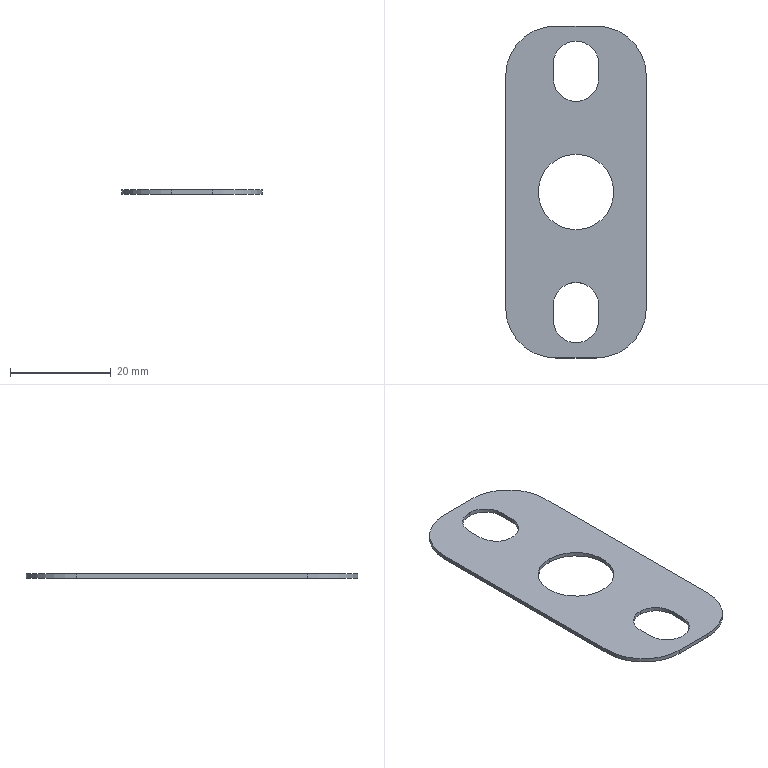Part | SolidWorks | features BaseBody 1 | 1 solid | 22 faces | box 28 x 66 x 0.8 mm | volume 1123 mm3 | cylinder 12 | plane 10 | commonest cylinder face diameters 9 x6 20 x4 15 x2
STEP:
#1=CARTESIAN_POINT('',(172.5,7.5,46.));
#2=VERTEX_POINT('',#1);
#3=CARTESIAN_POINT('',(172.5,-7.5,46.));
#4=VERTEX_POINT('',#3);
#5=CARTESIAN_POINT('',(172.5,0.,46.));
#6=DIRECTION('',(0.,0.,-1.));
#7=DIRECTION('',(0.,-1.,0.));
#8=AXIS2_PLACEMENT_3D('',#5,#6,#7);
#9=CIRCLE('',#8,7.5);
#10=EDGE_CURVE('',#2,#4,#9,.T.);
#11=ORIENTED_EDGE('',*,*,#10,.T.);
#12=CARTESIAN_POINT('',(172.5,-7.5,46.8));
#13=VERTEX_POINT('',#12);
#14=CARTESIAN_POINT('',(172.5,-7.5,46.));
#15=DIRECTION('',(0.,0.,1.));
#16=VECTOR('',#15,1000.);
#17=LINE('',#14,#16);
#18=EDGE_CURVE('',#4,#13,#17,.T.);
#19=ORIENTED_EDGE('',*,*,#18,.T.);
#20=CARTESIAN_POINT('',(172.5,7.5,46.8));
#21=VERTEX_POINT('',#20);
#22=CARTESIAN_POINT('',(172.5,0.,46.8));
#23=DIRECTION('',(0.,0.,-1.));
#24=DIRECTION('',(0.,-1.,0.));
#25=AXIS2_PLACEMENT_3D('',#22,#23,#24);
#26=CIRCLE('',#25,7.5);
#27=EDGE_CURVE('',#21,#13,#26,.T.);
#28=ORIENTED_EDGE('',*,*,#27,.F.);
#29=CARTESIAN_POINT('',(172.5,7.5,46.));
#30=DIRECTION('',(0.,0.,1.));
#31=VECTOR('',#30,1000.);
#32=LINE('',#29,#31);
#33=EDGE_CURVE('',#2,#21,#32,.T.);
#34=ORIENTED_EDGE('',*,*,#33,.F.);
#35=EDGE_LOOP('',(#11,#19,#28,#34));
#36=FACE_OUTER_BOUND('',#35,.T.);
#37=CARTESIAN_POINT('',(172.5,0.,46.));
#38=DIRECTION('',(0.,0.,1.));
#39=DIRECTION('',(0.,1.,0.));
#40=AXIS2_PLACEMENT_3D('',#37,#38,#39);
#41=CYLINDRICAL_SURFACE('',#40,7.5);
#42=ADVANCED_FACE('',(#36),#41,.F.);
#43=CARTESIAN_POINT('',(168.,25.5,46.));
#44=VERTEX_POINT('',#43);
#45=CARTESIAN_POINT('',(172.5,30.,46.));
#46=VERTEX_POINT('',#45);
#47=CARTESIAN_POINT('',(172.5,25.5,46.));
#48=DIRECTION('',(0.,0.,-1.));
#49=DIRECTION('',(0.,-1.,0.));
#50=AXIS2_PLACEMENT_3D('',#47,#48,#49);
#51=CIRCLE('',#50,4.5);
#52=EDGE_CURVE('',#44,#46,#51,.T.);
#53=ORIENTED_EDGE('',*,*,#52,.T.);
#54=CARTESIAN_POINT('',(172.5,30.,46.8));
#55=VERTEX_POINT('',#54);
#56=CARTESIAN_POINT('',(172.5,30.,46.));
#57=DIRECTION('',(0.,0.,1.));
#58=VECTOR('',#57,1000.);
#59=LINE('',#56,#58);
#60=EDGE_CURVE('',#46,#55,#59,.T.);
#61=ORIENTED_EDGE('',*,*,#60,.T.);
#62=CARTESIAN_POINT('',(168.,25.5,46.8));
#63=VERTEX_POINT('',#62);
#64=CARTESIAN_POINT('',(172.5,25.5,46.8));
#65=DIRECTION('',(0.,0.,-1.));
#66=DIRECTION('',(0.,-1.,0.));
#67=AXIS2_PLACEMENT_3D('',#64,#65,#66);
#68=CIRCLE('',#67,4.5);
#69=EDGE_CURVE('',#63,#55,#68,.T.);
#70=ORIENTED_EDGE('',*,*,#69,.F.);
#71=CARTESIAN_POINT('',(168.,25.5,46.));
#72=DIRECTION('',(0.,0.,1.));
#73=VECTOR('',#72,1000.);
#74=LINE('',#71,#73);
#75=EDGE_CURVE('',#44,#63,#74,.T.);
#76=ORIENTED_EDGE('',*,*,#75,.F.);
#77=EDGE_LOOP('',(#53,#61,#70,#76));
#78=FACE_OUTER_BOUND('',#77,.T.);
#79=CARTESIAN_POINT('',(172.5,25.5,46.));
#80=DIRECTION('',(0.,0.,1.));
#81=DIRECTION('',(0.,1.,0.));
#82=AXIS2_PLACEMENT_3D('',#79,#80,#81);
#83=CYLINDRICAL_SURFACE('',#82,4.5);
#84=ADVANCED_FACE('',(#78),#83,.F.);
#85=CARTESIAN_POINT('',(168.,-22.5,46.));
#86=VERTEX_POINT('',#85);
#87=CARTESIAN_POINT('',(172.5,-18.,46.));
#88=VERTEX_POINT('',#87);
#89=CARTESIAN_POINT('',(172.5,-22.5,46.));
#90=DIRECTION('',(0.,0.,-1.));
#91=DIRECTION('',(0.,1.,0.));
#92=AXIS2_PLACEMENT_3D('',#89,#90,#91);
#93=CIRCLE('',#92,4.5);
#94=EDGE_CURVE('',#86,#88,#93,.T.);
#95=ORIENTED_EDGE('',*,*,#94,.T.);
#96=CARTESIAN_POINT('',(172.5,-18.,46.8));
#97=VERTEX_POINT('',#96);
#98=CARTESIAN_POINT('',(172.5,-18.,46.));
#99=DIRECTION('',(0.,0.,1.));
#100=VECTOR('',#99,1000.);
#101=LINE('',#98,#100);
#102=EDGE_CURVE('',#88,#97,#101,.T.);
#103=ORIENTED_EDGE('',*,*,#102,.T.);
#104=CARTESIAN_POINT('',(168.,-22.5,46.8));
#105=VERTEX_POINT('',#104);
#106=CARTESIAN_POINT('',(172.5,-22.5,46.8));
#107=DIRECTION('',(0.,0.,-1.));
#108=DIRECTION('',(0.,1.,0.));
#109=AXIS2_PLACEMENT_3D('',#106,#107,#108);
#110=CIRCLE('',#109,4.5);
#111=EDGE_CURVE('',#105,#97,#110,.T.);
#112=ORIENTED_EDGE('',*,*,#111,.F.);
#113=CARTESIAN_POINT('',(168.,-22.5,46.));
#114=DIRECTION('',(0.,0.,1.));
#115=VECTOR('',#114,1000.);
#116=LINE('',#113,#115);
#117=EDGE_CURVE('',#86,#105,#116,.T.);
#118=ORIENTED_EDGE('',*,*,#117,.F.);
#119=EDGE_LOOP('',(#95,#103,#112,#118));
#120=FACE_OUTER_BOUND('',#119,.T.);
#121=CARTESIAN_POINT('',(172.5,-22.5,46.));
#122=DIRECTION('',(0.,0.,1.));
#123=DIRECTION('',(0.,1.,0.));
#124=AXIS2_PLACEMENT_3D('',#121,#122,#123);
#125=CYLINDRICAL_SURFACE('',#124,4.5);
#126=ADVANCED_FACE('',(#120),#125,.F.);
#127=CARTESIAN_POINT('',(177.,25.5,46.));
#128=VERTEX_POINT('',#127);
#129=CARTESIAN_POINT('',(177.,22.5,46.));
#130=VERTEX_POINT('',#129);
#131=CARTESIAN_POINT('',(177.,22.5,46.));
#132=DIRECTION('',(0.,-1.,0.));
#133=VECTOR('',#132,1000.);
#134=LINE('',#131,#133);
#135=EDGE_CURVE('',#128,#130,#134,.T.);
#136=ORIENTED_EDGE('',*,*,#135,.F.);
#137=CARTESIAN_POINT('',(172.5,25.5,46.));
#138=DIRECTION('',(0.,0.,-1.));
#139=DIRECTION('',(0.,-1.,0.));
#140=AXIS2_PLACEMENT_3D('',#137,#138,#139);
#141=CIRCLE('',#140,4.5);
#142=EDGE_CURVE('',#46,#128,#141,.T.);
#143=ORIENTED_EDGE('',*,*,#142,.F.);
#144=ORIENTED_EDGE('',*,*,#52,.F.);
#145=CARTESIAN_POINT('',(168.,22.5,46.));
#146=VERTEX_POINT('',#145);
#147=CARTESIAN_POINT('',(168.,25.5,46.));
#148=DIRECTION('',(0.,1.,0.));
#149=VECTOR('',#148,1000.);
#150=LINE('',#147,#149);
#151=EDGE_CURVE('',#146,#44,#150,.T.);
#152=ORIENTED_EDGE('',*,*,#151,.F.);
#153=CARTESIAN_POINT('',(172.5,22.5,46.));
#154=DIRECTION('',(0.,0.,-1.));
#155=DIRECTION('',(0.,-1.,0.));
#156=AXIS2_PLACEMENT_3D('',#153,#154,#155);
#157=CIRCLE('',#156,4.5);
#158=EDGE_CURVE('',#130,#146,#157,.T.);
#159=ORIENTED_EDGE('',*,*,#158,.F.);
#160=EDGE_LOOP('',(#136,#143,#144,#152,#159));
#161=FACE_BOUND('',#160,.T.);
#162=CARTESIAN_POINT('',(168.5,-33.,46.));
#163=VERTEX_POINT('',#162);
#164=CARTESIAN_POINT('',(158.5,-23.,46.));
#165=VERTEX_POINT('',#164);
#166=CARTESIAN_POINT('',(168.5,-23.,46.));
#167=DIRECTION('',(0.,0.,-1.));
#168=DIRECTION('',(0.,-1.,0.));
#169=AXIS2_PLACEMENT_3D('',#166,#167,#168);
#170=CIRCLE('',#169,10.);
#171=EDGE_CURVE('',#163,#165,#170,.T.);
#172=ORIENTED_EDGE('',*,*,#171,.T.);
#173=CARTESIAN_POINT('',(158.5,23.,46.));
#174=VERTEX_POINT('',#173);
#175=CARTESIAN_POINT('',(158.5,23.,46.));
#176=DIRECTION('',(0.,1.,0.));
#177=VECTOR('',#176,1000.);
#178=LINE('',#175,#177);
#179=EDGE_CURVE('',#165,#174,#178,.T.);
#180=ORIENTED_EDGE('',*,*,#179,.T.);
#181=CARTESIAN_POINT('',(168.5,33.,46.));
#182=VERTEX_POINT('',#181);
#183=CARTESIAN_POINT('',(168.5,23.,46.));
#184=DIRECTION('',(0.,0.,-1.));
#185=DIRECTION('',(0.,-1.,0.));
#186=AXIS2_PLACEMENT_3D('',#183,#184,#185);
#187=CIRCLE('',#186,10.);
#188=EDGE_CURVE('',#174,#182,#187,.T.);
#189=ORIENTED_EDGE('',*,*,#188,.T.);
#190=CARTESIAN_POINT('',(176.5,33.,46.));
#191=VERTEX_POINT('',#190);
#192=CARTESIAN_POINT('',(168.5,33.,46.));
#193=DIRECTION('',(1.,0.,0.));
#194=VECTOR('',#193,1000.);
#195=LINE('',#192,#194);
#196=EDGE_CURVE('',#182,#191,#195,.T.);
#197=ORIENTED_EDGE('',*,*,#196,.T.);
#198=CARTESIAN_POINT('',(186.5,23.,46.));
#199=VERTEX_POINT('',#198);
#200=CARTESIAN_POINT('',(176.5,23.,46.));
#201=DIRECTION('',(0.,0.,-1.));
#202=DIRECTION('',(0.,-1.,0.));
#203=AXIS2_PLACEMENT_3D('',#200,#201,#202);
#204=CIRCLE('',#203,10.);
#205=EDGE_CURVE('',#191,#199,#204,.T.);
#206=ORIENTED_EDGE('',*,*,#205,.T.);
#207=CARTESIAN_POINT('',(186.5,-23.,46.));
#208=VERTEX_POINT('',#207);
#209=CARTESIAN_POINT('',(186.5,23.,46.));
#210=DIRECTION('',(0.,-1.,0.));
#211=VECTOR('',#210,1000.);
#212=LINE('',#209,#211);
#213=EDGE_CURVE('',#199,#208,#212,.T.);
#214=ORIENTED_EDGE('',*,*,#213,.T.);
#215=CARTESIAN_POINT('',(176.5,-33.,46.));
#216=VERTEX_POINT('',#215);
#217=CARTESIAN_POINT('',(176.5,-23.,46.));
#218=DIRECTION('',(0.,0.,-1.));
#219=DIRECTION('',(0.,-1.,0.));
#220=AXIS2_PLACEMENT_3D('',#217,#218,#219);
#221=CIRCLE('',#220,10.);
#222=EDGE_CURVE('',#208,#216,#221,.T.);
#223=ORIENTED_EDGE('',*,*,#222,.T.);
#224=CARTESIAN_POINT('',(168.5,-33.,46.));
#225=DIRECTION('',(-1.,0.,0.));
#226=VECTOR('',#225,1000.);
#227=LINE('',#224,#226);
#228=EDGE_CURVE('',#216,#163,#227,.T.);
#229=ORIENTED_EDGE('',*,*,#228,.T.);
#230=EDGE_LOOP('',(#172,#180,#189,#197,#206,#214,#223,#229));
#231=FACE_OUTER_BOUND('',#230,.T.);
#232=CARTESIAN_POINT('',(177.,-22.5,46.));
#233=VERTEX_POINT('',#232);
#234=CARTESIAN_POINT('',(177.,-25.5,46.));
#235=VERTEX_POINT('',#234);
#236=CARTESIAN_POINT('',(177.,-22.5,46.));
#237=DIRECTION('',(0.,-1.,0.));
#238=VECTOR('',#237,1000.);
#239=LINE('',#236,#238);
#240=EDGE_CURVE('',#233,#235,#239,.T.);
#241=ORIENTED_EDGE('',*,*,#240,.F.);
#242=CARTESIAN_POINT('',(172.5,-22.5,46.));
#243=DIRECTION('',(0.,0.,-1.));
#244=DIRECTION('',(0.,1.,0.));
#245=AXIS2_PLACEMENT_3D('',#242,#243,#244);
#246=CIRCLE('',#245,4.5);
#247=EDGE_CURVE('',#88,#233,#246,.T.);
#248=ORIENTED_EDGE('',*,*,#247,.F.);
#249=ORIENTED_EDGE('',*,*,#94,.F.);
#250=CARTESIAN_POINT('',(168.,-25.5,46.));
#251=VERTEX_POINT('',#250);
#252=CARTESIAN_POINT('',(168.,-25.5,46.));
#253=DIRECTION('',(0.,1.,0.));
#254=VECTOR('',#253,1000.);
#255=LINE('',#252,#254);
#256=EDGE_CURVE('',#251,#86,#255,.T.);
#257=ORIENTED_EDGE('',*,*,#256,.F.);
#258=CARTESIAN_POINT('',(172.5,-25.5,46.));
#259=DIRECTION('',(0.,0.,-1.));
#260=DIRECTION('',(0.,1.,0.));
#261=AXIS2_PLACEMENT_3D('',#258,#259,#260);
#262=CIRCLE('',#261,4.5);
#263=EDGE_CURVE('',#235,#251,#262,.T.);
#264=ORIENTED_EDGE('',*,*,#263,.F.);
#265=EDGE_LOOP('',(#241,#248,#249,#257,#264));
#266=FACE_BOUND('',#265,.T.);
#267=ORIENTED_EDGE('',*,*,#10,.F.);
#268=CARTESIAN_POINT('',(172.5,0.,46.));
#269=DIRECTION('',(0.,0.,-1.));
#270=DIRECTION('',(0.,-1.,0.));
#271=AXIS2_PLACEMENT_3D('',#268,#269,#270);
#272=CIRCLE('',#271,7.5);
#273=EDGE_CURVE('',#4,#2,#272,.T.);
#274=ORIENTED_EDGE('',*,*,#273,.F.);
#275=EDGE_LOOP('',(#267,#274));
#276=FACE_BOUND('',#275,.T.);
#277=CARTESIAN_POINT('',(168.5,-23.,46.));
#278=DIRECTION('',(0.,0.,-1.));
#279=DIRECTION('',(0.,-1.,0.));
#280=AXIS2_PLACEMENT_3D('',#277,#278,#279);
#281=PLANE('',#280);
#282=ADVANCED_FACE('',(#161,#231,#266,#276),#281,.T.);
#283=ORIENTED_EDGE('',*,*,#69,.T.);
#284=CARTESIAN_POINT('',(177.,25.5,46.8));
#285=VERTEX_POINT('',#284);
#286=CARTESIAN_POINT('',(172.5,25.5,46.8));
#287=DIRECTION('',(0.,0.,-1.));
#288=DIRECTION('',(0.,-1.,0.));
#289=AXIS2_PLACEMENT_3D('',#286,#287,#288);
#290=CIRCLE('',#289,4.5);
#291=EDGE_CURVE('',#55,#285,#290,.T.);
#292=ORIENTED_EDGE('',*,*,#291,.T.);
#293=CARTESIAN_POINT('',(177.,22.5,46.8));
#294=VERTEX_POINT('',#293);
#295=CARTESIAN_POINT('',(177.,22.5,46.8));
#296=DIRECTION('',(0.,-1.,0.));
#297=VECTOR('',#296,1000.);
#298=LINE('',#295,#297);
#299=EDGE_CURVE('',#285,#294,#298,.T.);
#300=ORIENTED_EDGE('',*,*,#299,.T.);
#301=CARTESIAN_POINT('',(168.,22.5,46.8));
#302=VERTEX_POINT('',#301);
#303=CARTESIAN_POINT('',(172.5,22.5,46.8));
#304=DIRECTION('',(0.,0.,-1.));
#305=DIRECTION('',(0.,-1.,0.));
#306=AXIS2_PLACEMENT_3D('',#303,#304,#305);
#307=CIRCLE('',#306,4.5);
#308=EDGE_CURVE('',#294,#302,#307,.T.);
#309=ORIENTED_EDGE('',*,*,#308,.T.);
#310=CARTESIAN_POINT('',(168.,25.5,46.8));
#311=DIRECTION('',(0.,1.,0.));
#312=VECTOR('',#311,1000.);
#313=LINE('',#310,#312);
#314=EDGE_CURVE('',#302,#63,#313,.T.);
#315=ORIENTED_EDGE('',*,*,#314,.T.);
#316=EDGE_LOOP('',(#283,#292,#300,#309,#315));
#317=FACE_BOUND('',#316,.T.);
#318=CARTESIAN_POINT('',(168.5,-33.,46.8));
#319=VERTEX_POINT('',#318);
#320=CARTESIAN_POINT('',(158.5,-23.,46.8));
#321=VERTEX_POINT('',#320);
#322=CARTESIAN_POINT('',(168.5,-23.,46.8));
#323=DIRECTION('',(0.,0.,-1.));
#324=DIRECTION('',(0.,-1.,0.));
#325=AXIS2_PLACEMENT_3D('',#322,#323,#324);
#326=CIRCLE('',#325,10.);
#327=EDGE_CURVE('',#319,#321,#326,.T.);
#328=ORIENTED_EDGE('',*,*,#327,.F.);
#329=CARTESIAN_POINT('',(176.5,-33.,46.8));
#330=VERTEX_POINT('',#329);
#331=CARTESIAN_POINT('',(168.5,-33.,46.8));
#332=DIRECTION('',(-1.,0.,0.));
#333=VECTOR('',#332,1000.);
#334=LINE('',#331,#333);
#335=EDGE_CURVE('',#330,#319,#334,.T.);
#336=ORIENTED_EDGE('',*,*,#335,.F.);
#337=CARTESIAN_POINT('',(186.5,-23.,46.8));
#338=VERTEX_POINT('',#337);
#339=CARTESIAN_POINT('',(176.5,-23.,46.8));
#340=DIRECTION('',(0.,0.,-1.));
#341=DIRECTION('',(0.,-1.,0.));
#342=AXIS2_PLACEMENT_3D('',#339,#340,#341);
#343=CIRCLE('',#342,10.);
#344=EDGE_CURVE('',#338,#330,#343,.T.);
#345=ORIENTED_EDGE('',*,*,#344,.F.);
#346=CARTESIAN_POINT('',(186.5,23.,46.8));
#347=VERTEX_POINT('',#346);
#348=CARTESIAN_POINT('',(186.5,23.,46.8));
#349=DIRECTION('',(0.,-1.,0.));
#350=VECTOR('',#349,1000.);
#351=LINE('',#348,#350);
#352=EDGE_CURVE('',#347,#338,#351,.T.);
#353=ORIENTED_EDGE('',*,*,#352,.F.);
#354=CARTESIAN_POINT('',(176.5,33.,46.8));
#355=VERTEX_POINT('',#354);
#356=CARTESIAN_POINT('',(176.5,23.,46.8));
#357=DIRECTION('',(0.,0.,-1.));
#358=DIRECTION('',(0.,-1.,0.));
#359=AXIS2_PLACEMENT_3D('',#356,#357,#358);
#360=CIRCLE('',#359,10.);
#361=EDGE_CURVE('',#355,#347,#360,.T.);
#362=ORIENTED_EDGE('',*,*,#361,.F.);
#363=CARTESIAN_POINT('',(168.5,33.,46.8));
#364=VERTEX_POINT('',#363);
#365=CARTESIAN_POINT('',(168.5,33.,46.8));
#366=DIRECTION('',(1.,0.,0.));
#367=VECTOR('',#366,1000.);
#368=LINE('',#365,#367);
#369=EDGE_CURVE('',#364,#355,#368,.T.);
#370=ORIENTED_EDGE('',*,*,#369,.F.);
#371=CARTESIAN_POINT('',(158.5,23.,46.8));
#372=VERTEX_POINT('',#371);
#373=CARTESIAN_POINT('',(168.5,23.,46.8));
#374=DIRECTION('',(0.,0.,-1.));
#375=DIRECTION('',(0.,-1.,0.));
#376=AXIS2_PLACEMENT_3D('',#373,#374,#375);
#377=CIRCLE('',#376,10.);
#378=EDGE_CURVE('',#372,#364,#377,.T.);
#379=ORIENTED_EDGE('',*,*,#378,.F.);
#380=CARTESIAN_POINT('',(158.5,23.,46.8));
#381=DIRECTION('',(0.,1.,0.));
#382=VECTOR('',#381,1000.);
#383=LINE('',#380,#382);
#384=EDGE_CURVE('',#321,#372,#383,.T.);
#385=ORIENTED_EDGE('',*,*,#384,.F.);
#386=EDGE_LOOP('',(#328,#336,#345,#353,#362,#370,#379,#385));
#387=FACE_OUTER_BOUND('',#386,.T.);
#388=ORIENTED_EDGE('',*,*,#111,.T.);
#389=CARTESIAN_POINT('',(177.,-22.5,46.8));
#390=VERTEX_POINT('',#389);
#391=CARTESIAN_POINT('',(172.5,-22.5,46.8));
#392=DIRECTION('',(0.,0.,-1.));
#393=DIRECTION('',(0.,1.,0.));
#394=AXIS2_PLACEMENT_3D('',#391,#392,#393);
#395=CIRCLE('',#394,4.5);
#396=EDGE_CURVE('',#97,#390,#395,.T.);
#397=ORIENTED_EDGE('',*,*,#396,.T.);
#398=CARTESIAN_POINT('',(177.,-25.5,46.8));
#399=VERTEX_POINT('',#398);
#400=CARTESIAN_POINT('',(177.,-22.5,46.8));
#401=DIRECTION('',(0.,-1.,0.));
#402=VECTOR('',#401,1000.);
#403=LINE('',#400,#402);
#404=EDGE_CURVE('',#390,#399,#403,.T.);
#405=ORIENTED_EDGE('',*,*,#404,.T.);
#406=CARTESIAN_POINT('',(168.,-25.5,46.8));
#407=VERTEX_POINT('',#406);
#408=CARTESIAN_POINT('',(172.5,-25.5,46.8));
#409=DIRECTION('',(0.,0.,-1.));
#410=DIRECTION('',(0.,1.,0.));
#411=AXIS2_PLACEMENT_3D('',#408,#409,#410);
#412=CIRCLE('',#411,4.5);
#413=EDGE_CURVE('',#399,#407,#412,.T.);
#414=ORIENTED_EDGE('',*,*,#413,.T.);
#415=CARTESIAN_POINT('',(168.,-25.5,46.8));
#416=DIRECTION('',(0.,1.,0.));
#417=VECTOR('',#416,1000.);
#418=LINE('',#415,#417);
#419=EDGE_CURVE('',#407,#105,#418,.T.);
#420=ORIENTED_EDGE('',*,*,#419,.T.);
#421=EDGE_LOOP('',(#388,#397,#405,#414,#420));
#422=FACE_BOUND('',#421,.T.);
#423=ORIENTED_EDGE('',*,*,#27,.T.);
#424=CARTESIAN_POINT('',(172.5,0.,46.8));
#425=DIRECTION('',(0.,0.,-1.));
#426=DIRECTION('',(0.,-1.,0.));
#427=AXIS2_PLACEMENT_3D('',#424,#425,#426);
#428=CIRCLE('',#427,7.5);
#429=EDGE_CURVE('',#13,#21,#428,.T.);
#430=ORIENTED_EDGE('',*,*,#429,.T.);
#431=EDGE_LOOP('',(#423,#430));
#432=FACE_BOUND('',#431,.T.);
#433=CARTESIAN_POINT('',(168.5,-23.,46.8));
#434=DIRECTION('',(0.,0.,-1.));
#435=DIRECTION('',(0.,-1.,0.));
#436=AXIS2_PLACEMENT_3D('',#433,#434,#435);
#437=PLANE('',#436);
#438=ADVANCED_FACE('',(#317,#387,#422,#432),#437,.F.);
#439=ORIENTED_EDGE('',*,*,#327,.T.);
#440=CARTESIAN_POINT('',(158.5,-23.,46.));
#441=DIRECTION('',(0.,0.,1.));
#442=VECTOR('',#441,1000.);
#443=LINE('',#440,#442);
#444=EDGE_CURVE('',#165,#321,#443,.T.);
#445=ORIENTED_EDGE('',*,*,#444,.F.);
#446=ORIENTED_EDGE('',*,*,#171,.F.);
#447=CARTESIAN_POINT('',(168.5,-33.,46.));
#448=DIRECTION('',(0.,0.,1.));
#449=VECTOR('',#448,1000.);
#450=LINE('',#447,#449);
#451=EDGE_CURVE('',#163,#319,#450,.T.);
#452=ORIENTED_EDGE('',*,*,#451,.T.);
#453=EDGE_LOOP('',(#439,#445,#446,#452));
#454=FACE_OUTER_BOUND('',#453,.T.);
#455=CARTESIAN_POINT('',(168.5,-23.,46.));
#456=DIRECTION('',(0.,0.,1.));
#457=DIRECTION('',(0.,1.,0.));
#458=AXIS2_PLACEMENT_3D('',#455,#456,#457);
#459=CYLINDRICAL_SURFACE('',#458,10.);
#460=ADVANCED_FACE('',(#454),#459,.T.);
#461=ORIENTED_EDGE('',*,*,#384,.T.);
#462=CARTESIAN_POINT('',(158.5,23.,46.));
#463=DIRECTION('',(0.,0.,1.));
#464=VECTOR('',#463,1000.);
#465=LINE('',#462,#464);
#466=EDGE_CURVE('',#174,#372,#465,.T.);
#467=ORIENTED_EDGE('',*,*,#466,.F.);
#468=ORIENTED_EDGE('',*,*,#179,.F.);
#469=ORIENTED_EDGE('',*,*,#444,.T.);
#470=EDGE_LOOP('',(#461,#467,#468,#469));
#471=FACE_OUTER_BOUND('',#470,.T.);
#472=CARTESIAN_POINT('',(158.5,23.,46.));
#473=DIRECTION('',(1.,0.,0.));
#474=DIRECTION('',(0.,-1.,0.));
#475=AXIS2_PLACEMENT_3D('',#472,#473,#474);
#476=PLANE('',#475);
#477=ADVANCED_FACE('',(#471),#476,.F.);
#478=ORIENTED_EDGE('',*,*,#378,.T.);
#479=CARTESIAN_POINT('',(168.5,33.,46.));
#480=DIRECTION('',(0.,0.,1.));
#481=VECTOR('',#480,1000.);
#482=LINE('',#479,#481);
#483=EDGE_CURVE('',#182,#364,#482,.T.);
#484=ORIENTED_EDGE('',*,*,#483,.F.);
#485=ORIENTED_EDGE('',*,*,#188,.F.);
#486=ORIENTED_EDGE('',*,*,#466,.T.);
#487=EDGE_LOOP('',(#478,#484,#485,#486));
#488=FACE_OUTER_BOUND('',#487,.T.);
#489=CARTESIAN_POINT('',(168.5,23.,46.));
#490=DIRECTION('',(0.,0.,1.));
#491=DIRECTION('',(0.,1.,0.));
#492=AXIS2_PLACEMENT_3D('',#489,#490,#491);
#493=CYLINDRICAL_SURFACE('',#492,10.);
#494=ADVANCED_FACE('',(#488),#493,.T.);
#495=ORIENTED_EDGE('',*,*,#369,.T.);
#496=CARTESIAN_POINT('',(176.5,33.,46.));
#497=DIRECTION('',(0.,0.,1.));
#498=VECTOR('',#497,1000.);
#499=LINE('',#496,#498);
#500=EDGE_CURVE('',#191,#355,#499,.T.);
#501=ORIENTED_EDGE('',*,*,#500,.F.);
#502=ORIENTED_EDGE('',*,*,#196,.F.);
#503=ORIENTED_EDGE('',*,*,#483,.T.);
#504=EDGE_LOOP('',(#495,#501,#502,#503));
#505=FACE_OUTER_BOUND('',#504,.T.);
#506=CARTESIAN_POINT('',(168.5,33.,46.));
#507=DIRECTION('',(0.,-1.,0.));
#508=DIRECTION('',(0.,0.,1.));
#509=AXIS2_PLACEMENT_3D('',#506,#507,#508);
#510=PLANE('',#509);
#511=ADVANCED_FACE('',(#505),#510,.F.);
#512=ORIENTED_EDGE('',*,*,#361,.T.);
#513=CARTESIAN_POINT('',(186.5,23.,46.));
#514=DIRECTION('',(0.,0.,1.));
#515=VECTOR('',#514,1000.);
#516=LINE('',#513,#515);
#517=EDGE_CURVE('',#199,#347,#516,.T.);
#518=ORIENTED_EDGE('',*,*,#517,.F.);
#519=ORIENTED_EDGE('',*,*,#205,.F.);
#520=ORIENTED_EDGE('',*,*,#500,.T.);
#521=EDGE_LOOP('',(#512,#518,#519,#520));
#522=FACE_OUTER_BOUND('',#521,.T.);
#523=CARTESIAN_POINT('',(176.5,23.,46.));
#524=DIRECTION('',(0.,0.,1.));
#525=DIRECTION('',(0.,1.,0.));
#526=AXIS2_PLACEMENT_3D('',#523,#524,#525);
#527=CYLINDRICAL_SURFACE('',#526,10.);
#528=ADVANCED_FACE('',(#522),#527,.T.);
#529=ORIENTED_EDGE('',*,*,#352,.T.);
#530=CARTESIAN_POINT('',(186.5,-23.,46.));
#531=DIRECTION('',(0.,0.,1.));
#532=VECTOR('',#531,1000.);
#533=LINE('',#530,#532);
#534=EDGE_CURVE('',#208,#338,#533,.T.);
#535=ORIENTED_EDGE('',*,*,#534,.F.);
#536=ORIENTED_EDGE('',*,*,#213,.F.);
#537=ORIENTED_EDGE('',*,*,#517,.T.);
#538=EDGE_LOOP('',(#529,#535,#536,#537));
#539=FACE_OUTER_BOUND('',#538,.T.);
#540=CARTESIAN_POINT('',(186.5,23.,46.));
#541=DIRECTION('',(-1.,0.,0.));
#542=DIRECTION('',(0.,1.,0.));
#543=AXIS2_PLACEMENT_3D('',#540,#541,#542);
#544=PLANE('',#543);
#545=ADVANCED_FACE('',(#539),#544,.F.);
#546=ORIENTED_EDGE('',*,*,#344,.T.);
#547=CARTESIAN_POINT('',(176.5,-33.,46.));
#548=DIRECTION('',(0.,0.,1.));
#549=VECTOR('',#548,1000.);
#550=LINE('',#547,#549);
#551=EDGE_CURVE('',#216,#330,#550,.T.);
#552=ORIENTED_EDGE('',*,*,#551,.F.);
#553=ORIENTED_EDGE('',*,*,#222,.F.);
#554=ORIENTED_EDGE('',*,*,#534,.T.);
#555=EDGE_LOOP('',(#546,#552,#553,#554));
#556=FACE_OUTER_BOUND('',#555,.T.);
#557=CARTESIAN_POINT('',(176.5,-23.,46.));
#558=DIRECTION('',(0.,0.,1.));
#559=DIRECTION('',(0.,1.,0.));
#560=AXIS2_PLACEMENT_3D('',#557,#558,#559);
#561=CYLINDRICAL_SURFACE('',#560,10.);
#562=ADVANCED_FACE('',(#556),#561,.T.);
#563=ORIENTED_EDGE('',*,*,#335,.T.);
#564=ORIENTED_EDGE('',*,*,#451,.F.);
#565=ORIENTED_EDGE('',*,*,#228,.F.);
#566=ORIENTED_EDGE('',*,*,#551,.T.);
#567=EDGE_LOOP('',(#563,#564,#565,#566));
#568=FACE_OUTER_BOUND('',#567,.T.);
#569=CARTESIAN_POINT('',(168.5,-33.,46.));
#570=DIRECTION('',(0.,1.,0.));
#571=DIRECTION('',(0.,0.,-1.));
#572=AXIS2_PLACEMENT_3D('',#569,#570,#571);
#573=PLANE('',#572);
#574=ADVANCED_FACE('',(#568),#573,.F.);
#575=ORIENTED_EDGE('',*,*,#102,.F.);
#576=ORIENTED_EDGE('',*,*,#247,.T.);
#577=CARTESIAN_POINT('',(177.,-22.5,46.));
#578=DIRECTION('',(0.,0.,1.));
#579=VECTOR('',#578,1000.);
#580=LINE('',#577,#579);
#581=EDGE_CURVE('',#233,#390,#580,.T.);
#582=ORIENTED_EDGE('',*,*,#581,.T.);
#583=ORIENTED_EDGE('',*,*,#396,.F.);
#584=EDGE_LOOP('',(#575,#576,#582,#583));
#585=FACE_OUTER_BOUND('',#584,.T.);
#586=CARTESIAN_POINT('',(172.5,-22.5,46.));
#587=DIRECTION('',(0.,0.,1.));
#588=DIRECTION('',(0.,1.,0.));
#589=AXIS2_PLACEMENT_3D('',#586,#587,#588);
#590=CYLINDRICAL_SURFACE('',#589,4.5);
#591=ADVANCED_FACE('',(#585),#590,.F.);
#592=ORIENTED_EDGE('',*,*,#404,.F.);
#593=ORIENTED_EDGE('',*,*,#581,.F.);
#594=ORIENTED_EDGE('',*,*,#240,.T.);
#595=CARTESIAN_POINT('',(177.,-25.5,46.));
#596=DIRECTION('',(0.,0.,1.));
#597=VECTOR('',#596,1000.);
#598=LINE('',#595,#597);
#599=EDGE_CURVE('',#235,#399,#598,.T.);
#600=ORIENTED_EDGE('',*,*,#599,.T.);
#601=EDGE_LOOP('',(#592,#593,#594,#600));
#602=FACE_OUTER_BOUND('',#601,.T.);
#603=CARTESIAN_POINT('',(177.,-22.5,46.));
#604=DIRECTION('',(-1.,0.,0.));
#605=DIRECTION('',(0.,0.,-1.));
#606=AXIS2_PLACEMENT_3D('',#603,#604,#605);
#607=PLANE('',#606);
#608=ADVANCED_FACE('',(#602),#607,.T.);
#609=ORIENTED_EDGE('',*,*,#413,.F.);
#610=ORIENTED_EDGE('',*,*,#599,.F.);
#611=ORIENTED_EDGE('',*,*,#263,.T.);
#612=CARTESIAN_POINT('',(168.,-25.5,46.));
#613=DIRECTION('',(0.,0.,1.));
#614=VECTOR('',#613,1000.);
#615=LINE('',#612,#614);
#616=EDGE_CURVE('',#251,#407,#615,.T.);
#617=ORIENTED_EDGE('',*,*,#616,.T.);
#618=EDGE_LOOP('',(#609,#610,#611,#617));
#619=FACE_OUTER_BOUND('',#618,.T.);
#620=CARTESIAN_POINT('',(172.5,-25.5,46.));
#621=DIRECTION('',(0.,0.,1.));
#622=DIRECTION('',(0.,1.,0.));
#623=AXIS2_PLACEMENT_3D('',#620,#621,#622);
#624=CYLINDRICAL_SURFACE('',#623,4.5);
#625=ADVANCED_FACE('',(#619),#624,.F.);
#626=ORIENTED_EDGE('',*,*,#419,.F.);
#627=ORIENTED_EDGE('',*,*,#616,.F.);
#628=ORIENTED_EDGE('',*,*,#256,.T.);
#629=ORIENTED_EDGE('',*,*,#117,.T.);
#630=EDGE_LOOP('',(#626,#627,#628,#629));
#631=FACE_OUTER_BOUND('',#630,.T.);
#632=CARTESIAN_POINT('',(168.,-25.5,46.));
#633=DIRECTION('',(1.,0.,0.));
#634=DIRECTION('',(0.,0.,1.));
#635=AXIS2_PLACEMENT_3D('',#632,#633,#634);
#636=PLANE('',#635);
#637=ADVANCED_FACE('',(#631),#636,.T.);
#638=ORIENTED_EDGE('',*,*,#60,.F.);
#639=ORIENTED_EDGE('',*,*,#142,.T.);
#640=CARTESIAN_POINT('',(177.,25.5,46.));
#641=DIRECTION('',(0.,0.,1.));
#642=VECTOR('',#641,1000.);
#643=LINE('',#640,#642);
#644=EDGE_CURVE('',#128,#285,#643,.T.);
#645=ORIENTED_EDGE('',*,*,#644,.T.);
#646=ORIENTED_EDGE('',*,*,#291,.F.);
#647=EDGE_LOOP('',(#638,#639,#645,#646));
#648=FACE_OUTER_BOUND('',#647,.T.);
#649=CARTESIAN_POINT('',(172.5,25.5,46.));
#650=DIRECTION('',(0.,0.,1.));
#651=DIRECTION('',(0.,1.,0.));
#652=AXIS2_PLACEMENT_3D('',#649,#650,#651);
#653=CYLINDRICAL_SURFACE('',#652,4.5);
#654=ADVANCED_FACE('',(#648),#653,.F.);
#655=ORIENTED_EDGE('',*,*,#299,.F.);
#656=ORIENTED_EDGE('',*,*,#644,.F.);
#657=ORIENTED_EDGE('',*,*,#135,.T.);
#658=CARTESIAN_POINT('',(177.,22.5,46.));
#659=DIRECTION('',(0.,0.,1.));
#660=VECTOR('',#659,1000.);
#661=LINE('',#658,#660);
#662=EDGE_CURVE('',#130,#294,#661,.T.);
#663=ORIENTED_EDGE('',*,*,#662,.T.);
#664=EDGE_LOOP('',(#655,#656,#657,#663));
#665=FACE_OUTER_BOUND('',#664,.T.);
#666=CARTESIAN_POINT('',(177.,22.5,46.));
#667=DIRECTION('',(-1.,0.,0.));
#668=DIRECTION('',(0.,1.,0.));
#669=AXIS2_PLACEMENT_3D('',#666,#667,#668);
#670=PLANE('',#669);
#671=ADVANCED_FACE('',(#665),#670,.T.);
#672=ORIENTED_EDGE('',*,*,#308,.F.);
#673=ORIENTED_EDGE('',*,*,#662,.F.);
#674=ORIENTED_EDGE('',*,*,#158,.T.);
#675=CARTESIAN_POINT('',(168.,22.5,46.));
#676=DIRECTION('',(0.,0.,1.));
#677=VECTOR('',#676,1000.);
#678=LINE('',#675,#677);
#679=EDGE_CURVE('',#146,#302,#678,.T.);
#680=ORIENTED_EDGE('',*,*,#679,.T.);
#681=EDGE_LOOP('',(#672,#673,#674,#680));
#682=FACE_OUTER_BOUND('',#681,.T.);
#683=CARTESIAN_POINT('',(172.5,22.5,46.));
#684=DIRECTION('',(0.,0.,1.));
#685=DIRECTION('',(0.,1.,0.));
#686=AXIS2_PLACEMENT_3D('',#683,#684,#685);
#687=CYLINDRICAL_SURFACE('',#686,4.5);
#688=ADVANCED_FACE('',(#682),#687,.F.);
#689=ORIENTED_EDGE('',*,*,#314,.F.);
#690=ORIENTED_EDGE('',*,*,#679,.F.);
#691=ORIENTED_EDGE('',*,*,#151,.T.);
#692=ORIENTED_EDGE('',*,*,#75,.T.);
#693=EDGE_LOOP('',(#689,#690,#691,#692));
#694=FACE_OUTER_BOUND('',#693,.T.);
#695=CARTESIAN_POINT('',(168.,25.5,46.));
#696=DIRECTION('',(1.,0.,0.));
#697=DIRECTION('',(0.,-1.,0.));
#698=AXIS2_PLACEMENT_3D('',#695,#696,#697);
#699=PLANE('',#698);
#700=ADVANCED_FACE('',(#694),#699,.T.);
#701=ORIENTED_EDGE('',*,*,#18,.F.);
#702=ORIENTED_EDGE('',*,*,#273,.T.);
#703=ORIENTED_EDGE('',*,*,#33,.T.);
#704=ORIENTED_EDGE('',*,*,#429,.F.);
#705=EDGE_LOOP('',(#701,#702,#703,#704));
#706=FACE_OUTER_BOUND('',#705,.T.);
#707=CARTESIAN_POINT('',(172.5,0.,46.));
#708=DIRECTION('',(0.,0.,1.));
#709=DIRECTION('',(0.,1.,0.));
#710=AXIS2_PLACEMENT_3D('',#707,#708,#709);
#711=CYLINDRICAL_SURFACE('',#710,7.5);
#712=ADVANCED_FACE('',(#706),#711,.F.);
#713=CLOSED_SHELL('',(#42,#84,#126,#282,#438,#460,#477,#494,#511,#528,#545,#562,#574,#591,#608,#625,#637,#654,#671,#688,#700,#712));
#714=MANIFOLD_SOLID_BREP('',#713);
#715=CARTESIAN_POINT('',(0.,0.,0.));
#716=DIRECTION('',(0.,0.,1.));
#717=DIRECTION('',(1.,0.,0.));
#718=AXIS2_PLACEMENT_3D('',#715,#716,#717);
#719=(LENGTH_UNIT()NAMED_UNIT(*)SI_UNIT(.MILLI.,.METRE.));
#720=UNCERTAINTY_MEASURE_WITH_UNIT(LENGTH_MEASURE(0.00001),#719,'','');
#721=(NAMED_UNIT(*)PLANE_ANGLE_UNIT()SI_UNIT($,.RADIAN.));
#722=(NAMED_UNIT(*)SI_UNIT($,.STERADIAN.)SOLID_ANGLE_UNIT());
#723=(GEOMETRIC_REPRESENTATION_CONTEXT(3)GLOBAL_UNCERTAINTY_ASSIGNED_CONTEXT((#720))GLOBAL_UNIT_ASSIGNED_CONTEXT((#719,#721,#722))REPRESENTATION_CONTEXT('',''));
#724=ADVANCED_BREP_SHAPE_REPRESENTATION('',(#714,#718),#723);